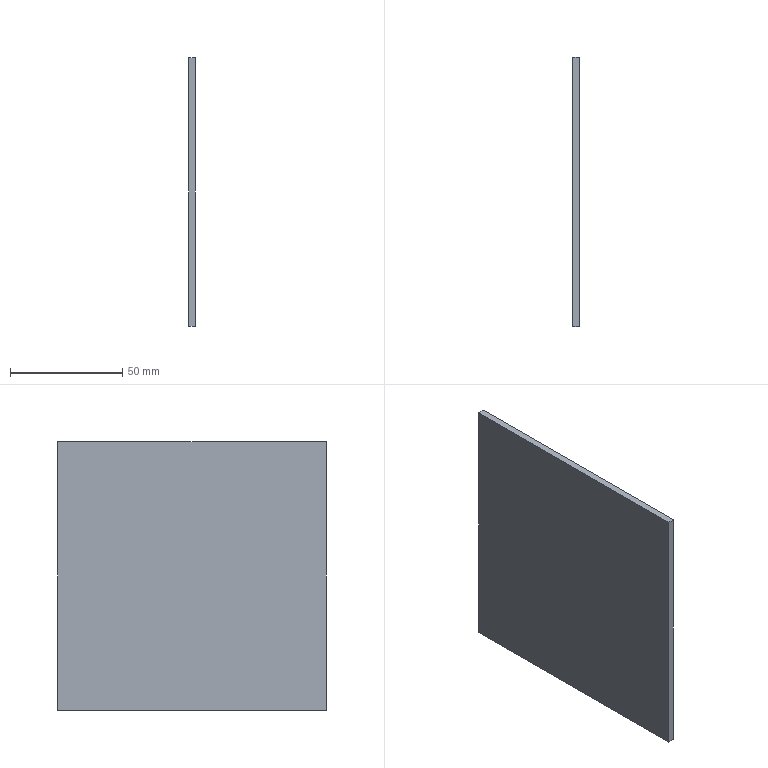Part | SolidWorks | 1 solid | 6 faces | box 3 x 120 x 120 mm | volume 43200 mm3 | plane 6
STEP:
#1=CARTESIAN_POINT('',(0.,60.,60.));
#2=VERTEX_POINT('',#1);
#3=CARTESIAN_POINT('',(0.,-60.,60.));
#4=VERTEX_POINT('',#3);
#5=CARTESIAN_POINT('',(0.,-60.,60.));
#6=DIRECTION('',(0.,-1.,0.));
#7=VECTOR('',#6,1000.);
#8=LINE('',#5,#7);
#9=EDGE_CURVE('',#2,#4,#8,.T.);
#10=ORIENTED_EDGE('',*,*,#9,.F.);
#11=CARTESIAN_POINT('',(-3.,60.,60.));
#12=VERTEX_POINT('',#11);
#13=CARTESIAN_POINT('',(-3.,60.,60.));
#14=DIRECTION('',(1.,0.,0.));
#15=VECTOR('',#14,1000.);
#16=LINE('',#13,#15);
#17=EDGE_CURVE('',#12,#2,#16,.T.);
#18=ORIENTED_EDGE('',*,*,#17,.F.);
#19=CARTESIAN_POINT('',(-3.,-60.,60.));
#20=VERTEX_POINT('',#19);
#21=CARTESIAN_POINT('',(-3.,-60.,60.));
#22=DIRECTION('',(0.,-1.,0.));
#23=VECTOR('',#22,1000.);
#24=LINE('',#21,#23);
#25=EDGE_CURVE('',#12,#20,#24,.T.);
#26=ORIENTED_EDGE('',*,*,#25,.T.);
#27=CARTESIAN_POINT('',(-3.,-60.,60.));
#28=DIRECTION('',(1.,0.,0.));
#29=VECTOR('',#28,1000.);
#30=LINE('',#27,#29);
#31=EDGE_CURVE('',#20,#4,#30,.T.);
#32=ORIENTED_EDGE('',*,*,#31,.T.);
#33=EDGE_LOOP('',(#10,#18,#26,#32));
#34=FACE_OUTER_BOUND('',#33,.T.);
#35=CARTESIAN_POINT('',(-3.,-60.,60.));
#36=DIRECTION('',(0.,0.,1.));
#37=DIRECTION('',(1.,0.,0.));
#38=AXIS2_PLACEMENT_3D('',#35,#36,#37);
#39=PLANE('',#38);
#40=ADVANCED_FACE('',(#34),#39,.T.);
#41=CARTESIAN_POINT('',(0.,60.,-60.));
#42=VERTEX_POINT('',#41);
#43=CARTESIAN_POINT('',(0.,60.,-60.));
#44=DIRECTION('',(0.,0.,1.));
#45=VECTOR('',#44,1000.);
#46=LINE('',#43,#45);
#47=EDGE_CURVE('',#42,#2,#46,.T.);
#48=ORIENTED_EDGE('',*,*,#47,.F.);
#49=CARTESIAN_POINT('',(-3.,60.,-60.));
#50=VERTEX_POINT('',#49);
#51=CARTESIAN_POINT('',(-3.,60.,-60.));
#52=DIRECTION('',(1.,0.,0.));
#53=VECTOR('',#52,1000.);
#54=LINE('',#51,#53);
#55=EDGE_CURVE('',#50,#42,#54,.T.);
#56=ORIENTED_EDGE('',*,*,#55,.F.);
#57=CARTESIAN_POINT('',(-3.,60.,-60.));
#58=DIRECTION('',(0.,0.,1.));
#59=VECTOR('',#58,1000.);
#60=LINE('',#57,#59);
#61=EDGE_CURVE('',#50,#12,#60,.T.);
#62=ORIENTED_EDGE('',*,*,#61,.T.);
#63=ORIENTED_EDGE('',*,*,#17,.T.);
#64=EDGE_LOOP('',(#48,#56,#62,#63));
#65=FACE_OUTER_BOUND('',#64,.T.);
#66=CARTESIAN_POINT('',(-3.,60.,-60.));
#67=DIRECTION('',(0.,1.,0.));
#68=DIRECTION('',(0.,0.,1.));
#69=AXIS2_PLACEMENT_3D('',#66,#67,#68);
#70=PLANE('',#69);
#71=ADVANCED_FACE('',(#65),#70,.T.);
#72=CARTESIAN_POINT('',(0.,-60.,-60.));
#73=VERTEX_POINT('',#72);
#74=CARTESIAN_POINT('',(0.,-60.,-60.));
#75=DIRECTION('',(0.,1.,0.));
#76=VECTOR('',#75,1000.);
#77=LINE('',#74,#76);
#78=EDGE_CURVE('',#73,#42,#77,.T.);
#79=ORIENTED_EDGE('',*,*,#78,.F.);
#80=CARTESIAN_POINT('',(-3.,-60.,-60.));
#81=VERTEX_POINT('',#80);
#82=CARTESIAN_POINT('',(-3.,-60.,-60.));
#83=DIRECTION('',(1.,0.,0.));
#84=VECTOR('',#83,1000.);
#85=LINE('',#82,#84);
#86=EDGE_CURVE('',#81,#73,#85,.T.);
#87=ORIENTED_EDGE('',*,*,#86,.F.);
#88=CARTESIAN_POINT('',(-3.,-60.,-60.));
#89=DIRECTION('',(0.,1.,0.));
#90=VECTOR('',#89,1000.);
#91=LINE('',#88,#90);
#92=EDGE_CURVE('',#81,#50,#91,.T.);
#93=ORIENTED_EDGE('',*,*,#92,.T.);
#94=ORIENTED_EDGE('',*,*,#55,.T.);
#95=EDGE_LOOP('',(#79,#87,#93,#94));
#96=FACE_OUTER_BOUND('',#95,.T.);
#97=CARTESIAN_POINT('',(-3.,-60.,-60.));
#98=DIRECTION('',(0.,0.,-1.));
#99=DIRECTION('',(-1.,0.,0.));
#100=AXIS2_PLACEMENT_3D('',#97,#98,#99);
#101=PLANE('',#100);
#102=ADVANCED_FACE('',(#96),#101,.T.);
#103=CARTESIAN_POINT('',(0.,-60.,-60.));
#104=DIRECTION('',(0.,0.,-1.));
#105=VECTOR('',#104,1000.);
#106=LINE('',#103,#105);
#107=EDGE_CURVE('',#4,#73,#106,.T.);
#108=ORIENTED_EDGE('',*,*,#107,.F.);
#109=ORIENTED_EDGE('',*,*,#31,.F.);
#110=CARTESIAN_POINT('',(-3.,-60.,-60.));
#111=DIRECTION('',(0.,0.,-1.));
#112=VECTOR('',#111,1000.);
#113=LINE('',#110,#112);
#114=EDGE_CURVE('',#20,#81,#113,.T.);
#115=ORIENTED_EDGE('',*,*,#114,.T.);
#116=ORIENTED_EDGE('',*,*,#86,.T.);
#117=EDGE_LOOP('',(#108,#109,#115,#116));
#118=FACE_OUTER_BOUND('',#117,.T.);
#119=CARTESIAN_POINT('',(-3.,-60.,-60.));
#120=DIRECTION('',(0.,-1.,0.));
#121=DIRECTION('',(0.,0.,-1.));
#122=AXIS2_PLACEMENT_3D('',#119,#120,#121);
#123=PLANE('',#122);
#124=ADVANCED_FACE('',(#118),#123,.T.);
#125=ORIENTED_EDGE('',*,*,#25,.F.);
#126=ORIENTED_EDGE('',*,*,#61,.F.);
#127=ORIENTED_EDGE('',*,*,#92,.F.);
#128=ORIENTED_EDGE('',*,*,#114,.F.);
#129=EDGE_LOOP('',(#125,#126,#127,#128));
#130=FACE_OUTER_BOUND('',#129,.T.);
#131=CARTESIAN_POINT('',(-3.,0.,0.));
#132=DIRECTION('',(1.,0.,0.));
#133=DIRECTION('',(0.,0.,-1.));
#134=AXIS2_PLACEMENT_3D('',#131,#132,#133);
#135=PLANE('',#134);
#136=ADVANCED_FACE('',(#130),#135,.F.);
#137=ORIENTED_EDGE('',*,*,#9,.T.);
#138=ORIENTED_EDGE('',*,*,#107,.T.);
#139=ORIENTED_EDGE('',*,*,#78,.T.);
#140=ORIENTED_EDGE('',*,*,#47,.T.);
#141=EDGE_LOOP('',(#137,#138,#139,#140));
#142=FACE_OUTER_BOUND('',#141,.T.);
#143=CARTESIAN_POINT('',(0.,0.,0.));
#144=DIRECTION('',(1.,0.,0.));
#145=DIRECTION('',(0.,0.,-1.));
#146=AXIS2_PLACEMENT_3D('',#143,#144,#145);
#147=PLANE('',#146);
#148=ADVANCED_FACE('',(#142),#147,.T.);
#149=CLOSED_SHELL('',(#40,#71,#102,#124,#136,#148));
#150=MANIFOLD_SOLID_BREP('',#149);
#151=CARTESIAN_POINT('',(0.,0.,0.));
#152=DIRECTION('',(0.,0.,1.));
#153=DIRECTION('',(1.,0.,0.));
#154=AXIS2_PLACEMENT_3D('',#151,#152,#153);
#155=(LENGTH_UNIT()NAMED_UNIT(*)SI_UNIT(.MILLI.,.METRE.));
#156=UNCERTAINTY_MEASURE_WITH_UNIT(LENGTH_MEASURE(0.00001),#155,'','');
#157=(NAMED_UNIT(*)PLANE_ANGLE_UNIT()SI_UNIT($,.RADIAN.));
#158=(NAMED_UNIT(*)SI_UNIT($,.STERADIAN.)SOLID_ANGLE_UNIT());
#159=(GEOMETRIC_REPRESENTATION_CONTEXT(3)GLOBAL_UNCERTAINTY_ASSIGNED_CONTEXT((#156))GLOBAL_UNIT_ASSIGNED_CONTEXT((#155,#157,#158))REPRESENTATION_CONTEXT('',''));
#160=ADVANCED_BREP_SHAPE_REPRESENTATION('',(#150,#154),#159);